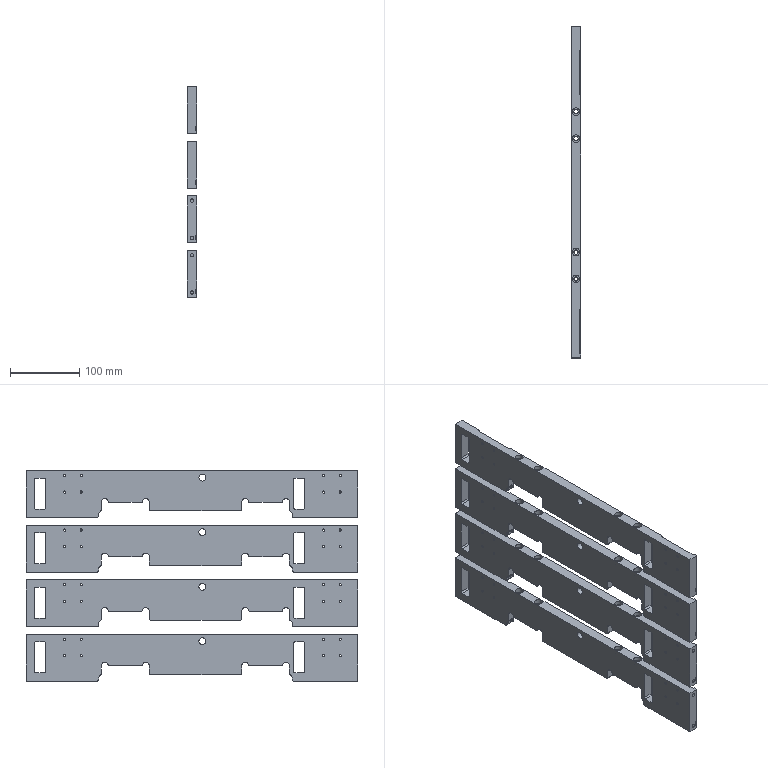CAM job | NX | 3+2 milling, drilling | part box 14 x 480 x 305 mm | stock box 14 x 485 x 310 mm
Tools:
number,name,description,diameter,corner_radius,flute_length,length,flutes
9,D10,平底铣刀-粗,10.0,0.0,35.0,75.0,2
11,D4-J,平底铣刀-精,4.0,0.0,50.0,75.0,2
7,D6-J,平底铣刀-精,6.0,0.0,25.0,75.0,2
1,D80R0.8飞刀,圆鼻刀-粗,80.0,0.8,50.0,75.0,2
2,D6倒角刀,倒角刀,6.0,0.0,3.0,25.0,2
21,M4X0.7,丝锥,3.3,0.0,35.0,50.0,2
13,ZT3.3,钻头,3.3,0.0,35.0,50.0,2
17,ZT10,钻头,10.0,0.0,35.0,50.0,2
Operations:
program,operation,operation_type,tool,method,geometry_group,spindle_rpm,surface_speed,feed_per_tooth,feed_cut,feed_plunge,cut_length_mm,path_length_mm,cut_time_min,machine_time_min
C,打点-深0.8_2,Operation,D6倒角刀,NONE,W-C,8000.0,150.796,0.0312,500.0,90.0,14.4,570.926,0.0288,0.0845
C,通孔-M4螺纹底孔_2,Operation,ZT3.3,NONE,W-C,3000.0,30.159,0.05,300.0,90.0,144.0,830.126,0.48,0.5486
C,钻倒角_3,Operation,D6倒角刀,METHOD,W-C,8000.0,150.796,0.0312,500.0,0.0,41.2,639.534,0.0824,0.1422
C,通孔-攻牙M4_2,Operation,M4X0.7,METHOD,W-C,600.0,6.22,0.0006,0.7,90.0,8.0,558.126,11.429,11.484
C,C0.3封闭铣廓倒角6X45L_COPY_1,PlanarMilling,D6倒角刀,爬面_倒角-切深0-步距G,W-C,7000.0,131.0,0.1071,1500.0,100.0,1492.47,2263.522,0.995,1.072
B,打点-深0.8,Operation,D6倒角刀,NONE,W-B,8000.0,150.796,0.0312,500.0,90.0,14.4,570.926,0.0288,0.0845
B,通孔-M4螺纹底孔,Operation,ZT3.3,NONE,W-B,3000.0,30.159,0.05,300.0,90.0,144.0,830.126,0.48,0.5486
B,钻倒角_2,Operation,D6倒角刀,METHOD,W-B,8000.0,150.796,0.0312,500.0,0.0,41.2,639.534,0.0824,0.1422
B,通孔-攻牙M4,Operation,M4X0.7,METHOD,W-B,600.0,6.22,0.0006,0.7,90.0,8.0,558.126,11.429,11.484
B,C0.3封闭铣廓倒角6X45L_COPY,PlanarMilling,D6倒角刀,爬面_倒角-切深0-步距G,W-B,7000.0,131.0,0.1071,1500.0,100.0,1491.198,2025.034,0.9941,1.048
A,面铣自动飞面精光_COPY,FaceMilling,D80R0.8飞刀,侧刃精光-切深K-步距G,W-A,4500.0,890.615,0.1111,1000.0,100.0,3663.0,3699.0,3.663,3.667
A,台阶粗_2,CavityMilling,D10,METHOD,W-A,8000.0,251.327,0.2188,3500.0,100.0,21336.828,23296.368,6.161,6.357
A,腰槽粗_1,VolumeBased25DMillingOperation,D10,METHOD,W-A,8000.0,251.327,0.1562,2500.0,100.0,19500.347,20775.762,7.8,7.928
A,打点,Operation,D6倒角刀,METHOD,W-A,3000.0,56.549,0.0333,200.0,0.0,90.0,1754.638,0.45,0.6165
A,打孔_2,Operation,ZT10,METHOD,W-A,1800.0,14.0,0.0333,120.0,0.0,58.0,396.019,0.4833,0.5171
A,清角D4,ZLevelMilling,D4-J,METHOD,W-A,6000.0,75.0,0.25,2500.0,80.0,16435.88,18511.311,6.578,6.785
A,底壁铣螺旋精光-中_COPY,VolumeBased25DMillingOperation,D4-J,螺旋精光-切深K-步距G,W-A,8000.0,100.528,0.05,800.0,100.0,2231.799,2677.917,2.79,2.834
A,外形粗_2,VolumeBased25DMillingOperation,D10,METHOD,W-A,6000.0,188.0,0.25,4000.0,80.0,139755.541,140200.546,34.939,34.983
A,底精_1,VolumeBased25DMillingOperation,D6-J,METHOD,W-A,6000.0,113.0,0.2083,1200.0,100.0,8570.297,9805.786,7.142,7.266
A,底侧精_3,VolumeBased25DMillingOperation,D6-J,METHOD,W-A,6000.0,113.0,0.2083,1200.0,100.0,1630.694,2874.426,1.359,1.483
A,腰槽精_1,VolumeBased25DMillingOperation,D6-J,METHOD,W-A,6000.0,113.0,0.0667,600.0,100.0,2405.48,3968.98,4.009,4.165
A,仅选体,SurfaceContour,D6倒角刀,METHOD,W-A,6000.0,113.0,0.125,1200.0,100.0,7420.541,12068.82,6.184,6.649
A,钻倒角_1,Operation,D6倒角刀,METHOD,W-A,5000.0,94.248,0.015,150.0,0.0,164.8,1728.586,1.099,1.255
A,铣倒角_1,PlanarMilling,D6倒角刀,METHOD,W-A,6000.0,113.097,0.05,600.0,100.0,125.097,536.801,0.2085,0.2497
A,外形半精_2,VolumeBased25DMillingOperation,D6-J,METHOD,W-A,6000.0,113.0,0.0833,1000.0,100.0,9630.06,10351.641,9.63,9.702
A,外形精_2,VolumeBased25DMillingOperation,D6-J,METHOD,W-A,6000.0,113.0,0.0833,1000.0,100.0,4814.23,5318.126,4.814,4.865